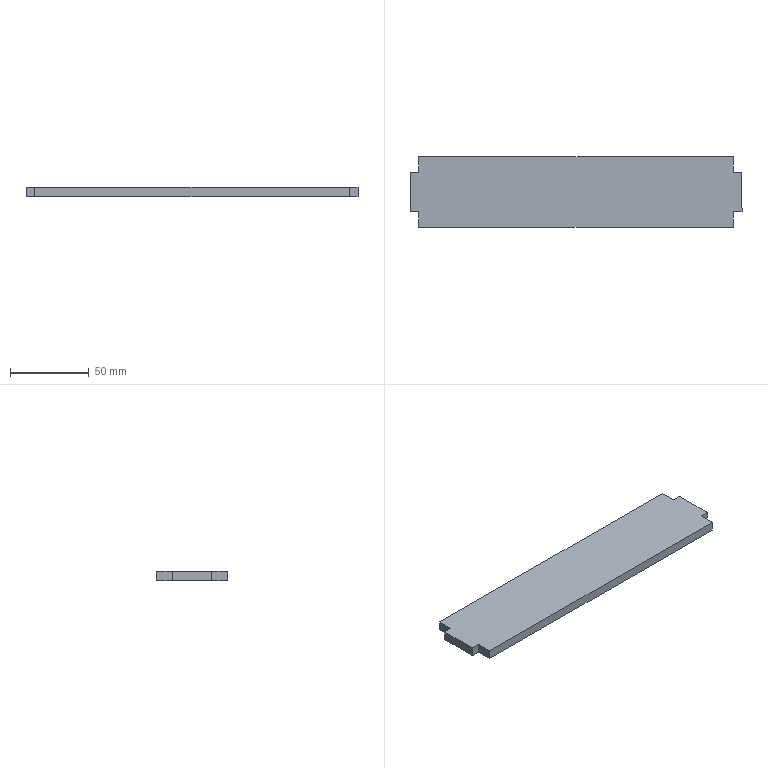Part | SolidWorks | features Extrusion 1 | 1 solid | 14 faces | box 211 x 45 x 6 mm | volume 55650 mm3 | plane 14
STEP:
#1=CARTESIAN_POINT('',(43.6,-110.,-3.));
#2=VERTEX_POINT('',#1);
#3=CARTESIAN_POINT('',(43.6,-100.,-3.));
#4=VERTEX_POINT('',#3);
#5=CARTESIAN_POINT('',(43.6,-100.,-3.));
#6=DIRECTION('',(0.,1.,0.));
#7=VECTOR('',#6,1000.);
#8=LINE('',#5,#7);
#9=EDGE_CURVE('',#2,#4,#8,.T.);
#10=ORIENTED_EDGE('',*,*,#9,.T.);
#11=CARTESIAN_POINT('',(43.6,-100.,3.));
#12=VERTEX_POINT('',#11);
#13=CARTESIAN_POINT('',(43.6,-100.,3.));
#14=DIRECTION('',(0.,0.,-1.));
#15=VECTOR('',#14,1000.);
#16=LINE('',#13,#15);
#17=EDGE_CURVE('',#12,#4,#16,.T.);
#18=ORIENTED_EDGE('',*,*,#17,.F.);
#19=CARTESIAN_POINT('',(43.6,-110.,3.));
#20=VERTEX_POINT('',#19);
#21=CARTESIAN_POINT('',(43.6,-100.,3.));
#22=DIRECTION('',(0.,1.,0.));
#23=VECTOR('',#22,1000.);
#24=LINE('',#21,#23);
#25=EDGE_CURVE('',#20,#12,#24,.T.);
#26=ORIENTED_EDGE('',*,*,#25,.F.);
#27=CARTESIAN_POINT('',(43.6,-110.,3.));
#28=DIRECTION('',(0.,0.,-1.));
#29=VECTOR('',#28,1000.);
#30=LINE('',#27,#29);
#31=EDGE_CURVE('',#20,#2,#30,.T.);
#32=ORIENTED_EDGE('',*,*,#31,.T.);
#33=EDGE_LOOP('',(#10,#18,#26,#32));
#34=FACE_OUTER_BOUND('',#33,.T.);
#35=CARTESIAN_POINT('',(43.6,-100.,3.));
#36=DIRECTION('',(-1.,0.,0.));
#37=DIRECTION('',(0.,-1.,0.));
#38=AXIS2_PLACEMENT_3D('',#35,#36,#37);
#39=PLANE('',#38);
#40=ADVANCED_FACE('',(#34),#39,.F.);
#41=CARTESIAN_POINT('',(49.1,-100.,-3.));
#42=VERTEX_POINT('',#41);
#43=CARTESIAN_POINT('',(43.6,-100.,-3.));
#44=DIRECTION('',(1.,0.,0.));
#45=VECTOR('',#44,1000.);
#46=LINE('',#43,#45);
#47=EDGE_CURVE('',#4,#42,#46,.T.);
#48=ORIENTED_EDGE('',*,*,#47,.T.);
#49=CARTESIAN_POINT('',(49.1,-100.,3.));
#50=VERTEX_POINT('',#49);
#51=CARTESIAN_POINT('',(49.1,-100.,3.));
#52=DIRECTION('',(0.,0.,-1.));
#53=VECTOR('',#52,1000.);
#54=LINE('',#51,#53);
#55=EDGE_CURVE('',#50,#42,#54,.T.);
#56=ORIENTED_EDGE('',*,*,#55,.F.);
#57=CARTESIAN_POINT('',(43.6,-100.,3.));
#58=DIRECTION('',(1.,0.,0.));
#59=VECTOR('',#58,1000.);
#60=LINE('',#57,#59);
#61=EDGE_CURVE('',#12,#50,#60,.T.);
#62=ORIENTED_EDGE('',*,*,#61,.F.);
#63=ORIENTED_EDGE('',*,*,#17,.T.);
#64=EDGE_LOOP('',(#48,#56,#62,#63));
#65=FACE_OUTER_BOUND('',#64,.T.);
#66=CARTESIAN_POINT('',(43.6,-100.,3.));
#67=DIRECTION('',(0.,1.,0.));
#68=DIRECTION('',(-1.,0.,0.));
#69=AXIS2_PLACEMENT_3D('',#66,#67,#68);
#70=PLANE('',#69);
#71=ADVANCED_FACE('',(#65),#70,.F.);
#72=CARTESIAN_POINT('',(49.1,-75.,-3.));
#73=VERTEX_POINT('',#72);
#74=CARTESIAN_POINT('',(49.1,-100.,-3.));
#75=DIRECTION('',(0.,1.,0.));
#76=VECTOR('',#75,1000.);
#77=LINE('',#74,#76);
#78=EDGE_CURVE('',#42,#73,#77,.T.);
#79=ORIENTED_EDGE('',*,*,#78,.T.);
#80=CARTESIAN_POINT('',(49.1,-75.,3.));
#81=VERTEX_POINT('',#80);
#82=CARTESIAN_POINT('',(49.1,-75.,3.));
#83=DIRECTION('',(0.,0.,-1.));
#84=VECTOR('',#83,1000.);
#85=LINE('',#82,#84);
#86=EDGE_CURVE('',#81,#73,#85,.T.);
#87=ORIENTED_EDGE('',*,*,#86,.F.);
#88=CARTESIAN_POINT('',(49.1,-100.,3.));
#89=DIRECTION('',(0.,1.,0.));
#90=VECTOR('',#89,1000.);
#91=LINE('',#88,#90);
#92=EDGE_CURVE('',#50,#81,#91,.T.);
#93=ORIENTED_EDGE('',*,*,#92,.F.);
#94=ORIENTED_EDGE('',*,*,#55,.T.);
#95=EDGE_LOOP('',(#79,#87,#93,#94));
#96=FACE_OUTER_BOUND('',#95,.T.);
#97=CARTESIAN_POINT('',(49.1,-100.,3.));
#98=DIRECTION('',(-1.,0.,0.));
#99=DIRECTION('',(0.,-1.,0.));
#100=AXIS2_PLACEMENT_3D('',#97,#98,#99);
#101=PLANE('',#100);
#102=ADVANCED_FACE('',(#96),#101,.F.);
#103=CARTESIAN_POINT('',(43.6,-75.,-3.));
#104=VERTEX_POINT('',#103);
#105=CARTESIAN_POINT('',(49.1,-75.,-3.));
#106=DIRECTION('',(-1.,0.,0.));
#107=VECTOR('',#106,1000.);
#108=LINE('',#105,#107);
#109=EDGE_CURVE('',#73,#104,#108,.T.);
#110=ORIENTED_EDGE('',*,*,#109,.T.);
#111=CARTESIAN_POINT('',(43.6,-75.,3.));
#112=VERTEX_POINT('',#111);
#113=CARTESIAN_POINT('',(43.6,-75.,3.));
#114=DIRECTION('',(0.,0.,-1.));
#115=VECTOR('',#114,1000.);
#116=LINE('',#113,#115);
#117=EDGE_CURVE('',#112,#104,#116,.T.);
#118=ORIENTED_EDGE('',*,*,#117,.F.);
#119=CARTESIAN_POINT('',(49.1,-75.,3.));
#120=DIRECTION('',(-1.,0.,0.));
#121=VECTOR('',#120,1000.);
#122=LINE('',#119,#121);
#123=EDGE_CURVE('',#81,#112,#122,.T.);
#124=ORIENTED_EDGE('',*,*,#123,.F.);
#125=ORIENTED_EDGE('',*,*,#86,.T.);
#126=EDGE_LOOP('',(#110,#118,#124,#125));
#127=FACE_OUTER_BOUND('',#126,.T.);
#128=CARTESIAN_POINT('',(49.1,-75.,3.));
#129=DIRECTION('',(0.,-1.,0.));
#130=DIRECTION('',(0.,0.,-1.));
#131=AXIS2_PLACEMENT_3D('',#128,#129,#130);
#132=PLANE('',#131);
#133=ADVANCED_FACE('',(#127),#132,.F.);
#134=CARTESIAN_POINT('',(43.6,-65.,-3.));
#135=VERTEX_POINT('',#134);
#136=CARTESIAN_POINT('',(43.6,-65.,-3.));
#137=DIRECTION('',(0.,1.,0.));
#138=VECTOR('',#137,1000.);
#139=LINE('',#136,#138);
#140=EDGE_CURVE('',#104,#135,#139,.T.);
#141=ORIENTED_EDGE('',*,*,#140,.T.);
#142=CARTESIAN_POINT('',(43.6,-65.,3.));
#143=VERTEX_POINT('',#142);
#144=CARTESIAN_POINT('',(43.6,-65.,3.));
#145=DIRECTION('',(0.,0.,-1.));
#146=VECTOR('',#145,1000.);
#147=LINE('',#144,#146);
#148=EDGE_CURVE('',#143,#135,#147,.T.);
#149=ORIENTED_EDGE('',*,*,#148,.F.);
#150=CARTESIAN_POINT('',(43.6,-65.,3.));
#151=DIRECTION('',(0.,1.,0.));
#152=VECTOR('',#151,1000.);
#153=LINE('',#150,#152);
#154=EDGE_CURVE('',#112,#143,#153,.T.);
#155=ORIENTED_EDGE('',*,*,#154,.F.);
#156=ORIENTED_EDGE('',*,*,#117,.T.);
#157=EDGE_LOOP('',(#141,#149,#155,#156));
#158=FACE_OUTER_BOUND('',#157,.T.);
#159=CARTESIAN_POINT('',(43.6,-65.,3.));
#160=DIRECTION('',(-1.,0.,0.));
#161=DIRECTION('',(0.,0.,1.));
#162=AXIS2_PLACEMENT_3D('',#159,#160,#161);
#163=PLANE('',#162);
#164=ADVANCED_FACE('',(#158),#163,.F.);
#165=CARTESIAN_POINT('',(-156.4,-65.,-3.));
#166=VERTEX_POINT('',#165);
#167=CARTESIAN_POINT('',(-156.4,-65.,-3.));
#168=DIRECTION('',(-1.,0.,0.));
#169=VECTOR('',#168,1000.);
#170=LINE('',#167,#169);
#171=EDGE_CURVE('',#135,#166,#170,.T.);
#172=ORIENTED_EDGE('',*,*,#171,.T.);
#173=CARTESIAN_POINT('',(-156.4,-65.,3.));
#174=VERTEX_POINT('',#173);
#175=CARTESIAN_POINT('',(-156.4,-65.,3.));
#176=DIRECTION('',(0.,0.,-1.));
#177=VECTOR('',#176,1000.);
#178=LINE('',#175,#177);
#179=EDGE_CURVE('',#174,#166,#178,.T.);
#180=ORIENTED_EDGE('',*,*,#179,.F.);
#181=CARTESIAN_POINT('',(-156.4,-65.,3.));
#182=DIRECTION('',(-1.,0.,0.));
#183=VECTOR('',#182,1000.);
#184=LINE('',#181,#183);
#185=EDGE_CURVE('',#143,#174,#184,.T.);
#186=ORIENTED_EDGE('',*,*,#185,.F.);
#187=ORIENTED_EDGE('',*,*,#148,.T.);
#188=EDGE_LOOP('',(#172,#180,#186,#187));
#189=FACE_OUTER_BOUND('',#188,.T.);
#190=CARTESIAN_POINT('',(-156.4,-65.,3.));
#191=DIRECTION('',(0.,-1.,0.));
#192=DIRECTION('',(0.,0.,-1.));
#193=AXIS2_PLACEMENT_3D('',#190,#191,#192);
#194=PLANE('',#193);
#195=ADVANCED_FACE('',(#189),#194,.F.);
#196=CARTESIAN_POINT('',(-156.4,-75.,-3.));
#197=VERTEX_POINT('',#196);
#198=CARTESIAN_POINT('',(-156.4,-75.,-3.));
#199=DIRECTION('',(0.,-1.,0.));
#200=VECTOR('',#199,1000.);
#201=LINE('',#198,#200);
#202=EDGE_CURVE('',#166,#197,#201,.T.);
#203=ORIENTED_EDGE('',*,*,#202,.T.);
#204=CARTESIAN_POINT('',(-156.4,-75.,3.));
#205=VERTEX_POINT('',#204);
#206=CARTESIAN_POINT('',(-156.4,-75.,3.));
#207=DIRECTION('',(0.,0.,-1.));
#208=VECTOR('',#207,1000.);
#209=LINE('',#206,#208);
#210=EDGE_CURVE('',#205,#197,#209,.T.);
#211=ORIENTED_EDGE('',*,*,#210,.F.);
#212=CARTESIAN_POINT('',(-156.4,-75.,3.));
#213=DIRECTION('',(0.,-1.,0.));
#214=VECTOR('',#213,1000.);
#215=LINE('',#212,#214);
#216=EDGE_CURVE('',#174,#205,#215,.T.);
#217=ORIENTED_EDGE('',*,*,#216,.F.);
#218=ORIENTED_EDGE('',*,*,#179,.T.);
#219=EDGE_LOOP('',(#203,#211,#217,#218));
#220=FACE_OUTER_BOUND('',#219,.T.);
#221=CARTESIAN_POINT('',(-156.4,-75.,3.));
#222=DIRECTION('',(1.,0.,0.));
#223=DIRECTION('',(0.,0.,-1.));
#224=AXIS2_PLACEMENT_3D('',#221,#222,#223);
#225=PLANE('',#224);
#226=ADVANCED_FACE('',(#220),#225,.F.);
#227=CARTESIAN_POINT('',(-161.9,-75.,-3.));
#228=VERTEX_POINT('',#227);
#229=CARTESIAN_POINT('',(-161.9,-75.,-3.));
#230=DIRECTION('',(-1.,0.,0.));
#231=VECTOR('',#230,1000.);
#232=LINE('',#229,#231);
#233=EDGE_CURVE('',#197,#228,#232,.T.);
#234=ORIENTED_EDGE('',*,*,#233,.T.);
#235=CARTESIAN_POINT('',(-161.9,-75.,3.));
#236=VERTEX_POINT('',#235);
#237=CARTESIAN_POINT('',(-161.9,-75.,3.));
#238=DIRECTION('',(0.,0.,-1.));
#239=VECTOR('',#238,1000.);
#240=LINE('',#237,#239);
#241=EDGE_CURVE('',#236,#228,#240,.T.);
#242=ORIENTED_EDGE('',*,*,#241,.F.);
#243=CARTESIAN_POINT('',(-161.9,-75.,3.));
#244=DIRECTION('',(-1.,0.,0.));
#245=VECTOR('',#244,1000.);
#246=LINE('',#243,#245);
#247=EDGE_CURVE('',#205,#236,#246,.T.);
#248=ORIENTED_EDGE('',*,*,#247,.F.);
#249=ORIENTED_EDGE('',*,*,#210,.T.);
#250=EDGE_LOOP('',(#234,#242,#248,#249));
#251=FACE_OUTER_BOUND('',#250,.T.);
#252=CARTESIAN_POINT('',(-161.9,-75.,3.));
#253=DIRECTION('',(0.,-1.,0.));
#254=DIRECTION('',(1.,0.,0.));
#255=AXIS2_PLACEMENT_3D('',#252,#253,#254);
#256=PLANE('',#255);
#257=ADVANCED_FACE('',(#251),#256,.F.);
#258=CARTESIAN_POINT('',(-161.9,-100.,-3.));
#259=VERTEX_POINT('',#258);
#260=CARTESIAN_POINT('',(-161.9,-100.,-3.));
#261=DIRECTION('',(0.,-1.,0.));
#262=VECTOR('',#261,1000.);
#263=LINE('',#260,#262);
#264=EDGE_CURVE('',#228,#259,#263,.T.);
#265=ORIENTED_EDGE('',*,*,#264,.T.);
#266=CARTESIAN_POINT('',(-161.9,-100.,3.));
#267=VERTEX_POINT('',#266);
#268=CARTESIAN_POINT('',(-161.9,-100.,3.));
#269=DIRECTION('',(0.,0.,-1.));
#270=VECTOR('',#269,1000.);
#271=LINE('',#268,#270);
#272=EDGE_CURVE('',#267,#259,#271,.T.);
#273=ORIENTED_EDGE('',*,*,#272,.F.);
#274=CARTESIAN_POINT('',(-161.9,-100.,3.));
#275=DIRECTION('',(0.,-1.,0.));
#276=VECTOR('',#275,1000.);
#277=LINE('',#274,#276);
#278=EDGE_CURVE('',#236,#267,#277,.T.);
#279=ORIENTED_EDGE('',*,*,#278,.F.);
#280=ORIENTED_EDGE('',*,*,#241,.T.);
#281=EDGE_LOOP('',(#265,#273,#279,#280));
#282=FACE_OUTER_BOUND('',#281,.T.);
#283=CARTESIAN_POINT('',(-161.9,-100.,3.));
#284=DIRECTION('',(1.,0.,0.));
#285=DIRECTION('',(0.,0.,-1.));
#286=AXIS2_PLACEMENT_3D('',#283,#284,#285);
#287=PLANE('',#286);
#288=ADVANCED_FACE('',(#282),#287,.F.);
#289=CARTESIAN_POINT('',(-156.4,-100.,-3.));
#290=VERTEX_POINT('',#289);
#291=CARTESIAN_POINT('',(-156.4,-100.,-3.));
#292=DIRECTION('',(1.,0.,0.));
#293=VECTOR('',#292,1000.);
#294=LINE('',#291,#293);
#295=EDGE_CURVE('',#259,#290,#294,.T.);
#296=ORIENTED_EDGE('',*,*,#295,.T.);
#297=CARTESIAN_POINT('',(-156.4,-100.,3.));
#298=VERTEX_POINT('',#297);
#299=CARTESIAN_POINT('',(-156.4,-100.,3.));
#300=DIRECTION('',(0.,0.,-1.));
#301=VECTOR('',#300,1000.);
#302=LINE('',#299,#301);
#303=EDGE_CURVE('',#298,#290,#302,.T.);
#304=ORIENTED_EDGE('',*,*,#303,.F.);
#305=CARTESIAN_POINT('',(-156.4,-100.,3.));
#306=DIRECTION('',(1.,0.,0.));
#307=VECTOR('',#306,1000.);
#308=LINE('',#305,#307);
#309=EDGE_CURVE('',#267,#298,#308,.T.);
#310=ORIENTED_EDGE('',*,*,#309,.F.);
#311=ORIENTED_EDGE('',*,*,#272,.T.);
#312=EDGE_LOOP('',(#296,#304,#310,#311));
#313=FACE_OUTER_BOUND('',#312,.T.);
#314=CARTESIAN_POINT('',(-156.4,-100.,3.));
#315=DIRECTION('',(0.,1.,0.));
#316=DIRECTION('',(-1.,0.,0.));
#317=AXIS2_PLACEMENT_3D('',#314,#315,#316);
#318=PLANE('',#317);
#319=ADVANCED_FACE('',(#313),#318,.F.);
#320=CARTESIAN_POINT('',(-156.4,-110.,-3.));
#321=VERTEX_POINT('',#320);
#322=CARTESIAN_POINT('',(-156.4,-110.,-3.));
#323=DIRECTION('',(0.,-1.,0.));
#324=VECTOR('',#323,1000.);
#325=LINE('',#322,#324);
#326=EDGE_CURVE('',#290,#321,#325,.T.);
#327=ORIENTED_EDGE('',*,*,#326,.T.);
#328=CARTESIAN_POINT('',(-156.4,-110.,3.));
#329=VERTEX_POINT('',#328);
#330=CARTESIAN_POINT('',(-156.4,-110.,3.));
#331=DIRECTION('',(0.,0.,-1.));
#332=VECTOR('',#331,1000.);
#333=LINE('',#330,#332);
#334=EDGE_CURVE('',#329,#321,#333,.T.);
#335=ORIENTED_EDGE('',*,*,#334,.F.);
#336=CARTESIAN_POINT('',(-156.4,-110.,3.));
#337=DIRECTION('',(0.,-1.,0.));
#338=VECTOR('',#337,1000.);
#339=LINE('',#336,#338);
#340=EDGE_CURVE('',#298,#329,#339,.T.);
#341=ORIENTED_EDGE('',*,*,#340,.F.);
#342=ORIENTED_EDGE('',*,*,#303,.T.);
#343=EDGE_LOOP('',(#327,#335,#341,#342));
#344=FACE_OUTER_BOUND('',#343,.T.);
#345=CARTESIAN_POINT('',(-156.4,-110.,3.));
#346=DIRECTION('',(1.,0.,0.));
#347=DIRECTION('',(0.,0.,-1.));
#348=AXIS2_PLACEMENT_3D('',#345,#346,#347);
#349=PLANE('',#348);
#350=ADVANCED_FACE('',(#344),#349,.F.);
#351=CARTESIAN_POINT('',(43.6,-110.,-3.));
#352=DIRECTION('',(1.,0.,0.));
#353=VECTOR('',#352,1000.);
#354=LINE('',#351,#353);
#355=EDGE_CURVE('',#321,#2,#354,.T.);
#356=ORIENTED_EDGE('',*,*,#355,.T.);
#357=ORIENTED_EDGE('',*,*,#31,.F.);
#358=CARTESIAN_POINT('',(43.6,-110.,3.));
#359=DIRECTION('',(1.,0.,0.));
#360=VECTOR('',#359,1000.);
#361=LINE('',#358,#360);
#362=EDGE_CURVE('',#329,#20,#361,.T.);
#363=ORIENTED_EDGE('',*,*,#362,.F.);
#364=ORIENTED_EDGE('',*,*,#334,.T.);
#365=EDGE_LOOP('',(#356,#357,#363,#364));
#366=FACE_OUTER_BOUND('',#365,.T.);
#367=CARTESIAN_POINT('',(43.6,-110.,3.));
#368=DIRECTION('',(0.,1.,0.));
#369=DIRECTION('',(0.,0.,1.));
#370=AXIS2_PLACEMENT_3D('',#367,#368,#369);
#371=PLANE('',#370);
#372=ADVANCED_FACE('',(#366),#371,.F.);
#373=ORIENTED_EDGE('',*,*,#25,.T.);
#374=ORIENTED_EDGE('',*,*,#61,.T.);
#375=ORIENTED_EDGE('',*,*,#92,.T.);
#376=ORIENTED_EDGE('',*,*,#123,.T.);
#377=ORIENTED_EDGE('',*,*,#154,.T.);
#378=ORIENTED_EDGE('',*,*,#185,.T.);
#379=ORIENTED_EDGE('',*,*,#216,.T.);
#380=ORIENTED_EDGE('',*,*,#247,.T.);
#381=ORIENTED_EDGE('',*,*,#278,.T.);
#382=ORIENTED_EDGE('',*,*,#309,.T.);
#383=ORIENTED_EDGE('',*,*,#340,.T.);
#384=ORIENTED_EDGE('',*,*,#362,.T.);
#385=EDGE_LOOP('',(#373,#374,#375,#376,#377,#378,#379,#380,#381,#382,#383,#384));
#386=FACE_OUTER_BOUND('',#385,.T.);
#387=CARTESIAN_POINT('',(0.,0.,3.));
#388=DIRECTION('',(0.,0.,-1.));
#389=DIRECTION('',(-1.,0.,0.));
#390=AXIS2_PLACEMENT_3D('',#387,#388,#389);
#391=PLANE('',#390);
#392=ADVANCED_FACE('',(#386),#391,.F.);
#393=ORIENTED_EDGE('',*,*,#9,.F.);
#394=ORIENTED_EDGE('',*,*,#355,.F.);
#395=ORIENTED_EDGE('',*,*,#326,.F.);
#396=ORIENTED_EDGE('',*,*,#295,.F.);
#397=ORIENTED_EDGE('',*,*,#264,.F.);
#398=ORIENTED_EDGE('',*,*,#233,.F.);
#399=ORIENTED_EDGE('',*,*,#202,.F.);
#400=ORIENTED_EDGE('',*,*,#171,.F.);
#401=ORIENTED_EDGE('',*,*,#140,.F.);
#402=ORIENTED_EDGE('',*,*,#109,.F.);
#403=ORIENTED_EDGE('',*,*,#78,.F.);
#404=ORIENTED_EDGE('',*,*,#47,.F.);
#405=EDGE_LOOP('',(#393,#394,#395,#396,#397,#398,#399,#400,#401,#402,#403,#404));
#406=FACE_OUTER_BOUND('',#405,.T.);
#407=CARTESIAN_POINT('',(0.,0.,-3.));
#408=DIRECTION('',(0.,0.,-1.));
#409=DIRECTION('',(-1.,0.,0.));
#410=AXIS2_PLACEMENT_3D('',#407,#408,#409);
#411=PLANE('',#410);
#412=ADVANCED_FACE('',(#406),#411,.T.);
#413=CLOSED_SHELL('',(#40,#71,#102,#133,#164,#195,#226,#257,#288,#319,#350,#372,#392,#412));
#414=MANIFOLD_SOLID_BREP('',#413);
#415=CARTESIAN_POINT('',(0.,0.,0.));
#416=DIRECTION('',(0.,0.,1.));
#417=DIRECTION('',(1.,0.,0.));
#418=AXIS2_PLACEMENT_3D('',#415,#416,#417);
#419=(LENGTH_UNIT()NAMED_UNIT(*)SI_UNIT(.MILLI.,.METRE.));
#420=UNCERTAINTY_MEASURE_WITH_UNIT(LENGTH_MEASURE(0.00001),#419,'','');
#421=(NAMED_UNIT(*)PLANE_ANGLE_UNIT()SI_UNIT($,.RADIAN.));
#422=(NAMED_UNIT(*)SI_UNIT($,.STERADIAN.)SOLID_ANGLE_UNIT());
#423=(GEOMETRIC_REPRESENTATION_CONTEXT(3)GLOBAL_UNCERTAINTY_ASSIGNED_CONTEXT((#420))GLOBAL_UNIT_ASSIGNED_CONTEXT((#419,#421,#422))REPRESENTATION_CONTEXT('',''));
#424=ADVANCED_BREP_SHAPE_REPRESENTATION('',(#414,#418),#423);